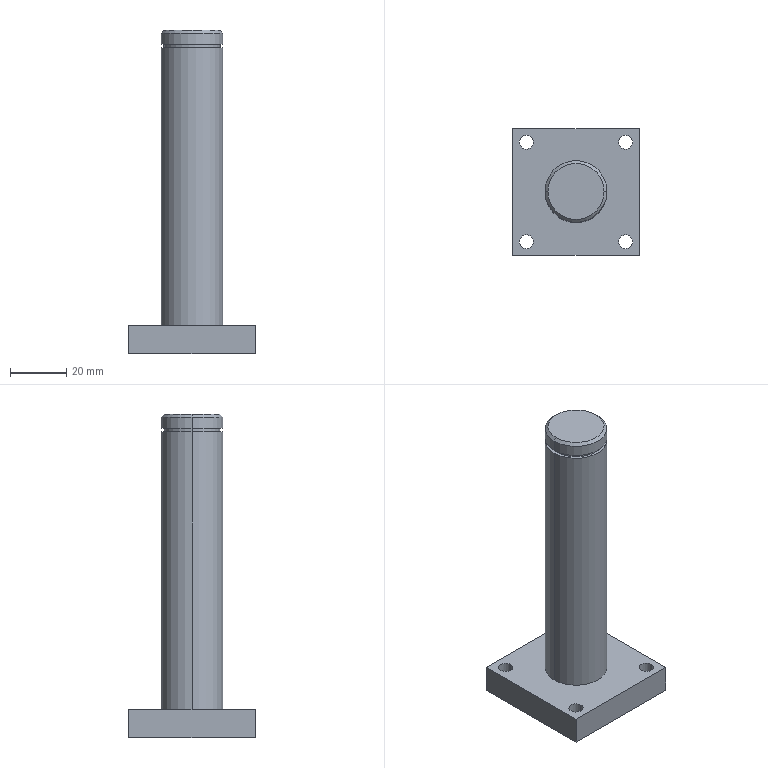Part | SolidWorks | features ICE 2, Chamfer 1, Extrusion 1 | 1 solid | 25 faces | box 45 x 45 x 115 mm | volume 59266 mm3 | cylinder 14 | plane 9 | cone 2 | commonest cylinder face diameters 5 x8 22 x4 20 x2
STEP:
#1=CARTESIAN_POINT('',(-11.,0.,114.));
#2=VERTEX_POINT('',#1);
#3=CARTESIAN_POINT('',(11.,0.,114.));
#4=VERTEX_POINT('',#3);
#5=CARTESIAN_POINT('',(0.,0.,114.));
#6=DIRECTION('',(0.,0.,-1.));
#7=DIRECTION('',(1.,0.,0.));
#8=AXIS2_PLACEMENT_3D('',#5,#6,#7);
#9=CIRCLE('',#8,11.);
#10=EDGE_CURVE('',#2,#4,#9,.T.);
#11=ORIENTED_EDGE('',*,*,#10,.T.);
#12=CARTESIAN_POINT('',(11.,0.,110.));
#13=VERTEX_POINT('',#12);
#14=CARTESIAN_POINT('',(11.,0.,115.));
#15=DIRECTION('',(0.,0.,-1.));
#16=VECTOR('',#15,1000.);
#17=LINE('',#14,#16);
#18=EDGE_CURVE('',#4,#13,#17,.T.);
#19=ORIENTED_EDGE('',*,*,#18,.T.);
#20=CARTESIAN_POINT('',(-11.,0.,110.));
#21=VERTEX_POINT('',#20);
#22=CARTESIAN_POINT('',(0.,0.,110.));
#23=DIRECTION('',(0.,0.,1.));
#24=DIRECTION('',(1.,0.,0.));
#25=AXIS2_PLACEMENT_3D('',#22,#23,#24);
#26=CIRCLE('',#25,11.);
#27=EDGE_CURVE('',#13,#21,#26,.T.);
#28=ORIENTED_EDGE('',*,*,#27,.T.);
#29=CARTESIAN_POINT('',(-11.,0.,115.));
#30=DIRECTION('',(0.,0.,-1.));
#31=VECTOR('',#30,1000.);
#32=LINE('',#29,#31);
#33=EDGE_CURVE('',#2,#21,#32,.T.);
#34=ORIENTED_EDGE('',*,*,#33,.F.);
#35=EDGE_LOOP('',(#11,#19,#28,#34));
#36=FACE_OUTER_BOUND('',#35,.T.);
#37=CARTESIAN_POINT('',(0.,0.,115.));
#38=DIRECTION('',(0.,0.,-1.));
#39=DIRECTION('',(-1.,0.,0.));
#40=AXIS2_PLACEMENT_3D('',#37,#38,#39);
#41=CYLINDRICAL_SURFACE('',#40,11.);
#42=ADVANCED_FACE('',(#36),#41,.T.);
#43=CARTESIAN_POINT('',(10.,0.,115.));
#44=VERTEX_POINT('',#43);
#45=CARTESIAN_POINT('',(-10.,0.,115.));
#46=VERTEX_POINT('',#45);
#47=CARTESIAN_POINT('',(0.,0.,115.));
#48=DIRECTION('',(0.,0.,1.));
#49=DIRECTION('',(1.,0.,0.));
#50=AXIS2_PLACEMENT_3D('',#47,#48,#49);
#51=CIRCLE('',#50,10.);
#52=EDGE_CURVE('',#44,#46,#51,.T.);
#53=ORIENTED_EDGE('',*,*,#52,.F.);
#54=CARTESIAN_POINT('',(10.,0.,115.));
#55=DIRECTION('',(0.7071,0.,-0.7071));
#56=VECTOR('',#55,1000.);
#57=LINE('',#54,#56);
#58=EDGE_CURVE('',#44,#4,#57,.T.);
#59=ORIENTED_EDGE('',*,*,#58,.T.);
#60=ORIENTED_EDGE('',*,*,#10,.F.);
#61=CARTESIAN_POINT('',(-10.,0.,115.));
#62=DIRECTION('',(-0.7071,0.,-0.7071));
#63=VECTOR('',#62,1000.);
#64=LINE('',#61,#63);
#65=EDGE_CURVE('',#46,#2,#64,.T.);
#66=ORIENTED_EDGE('',*,*,#65,.F.);
#67=EDGE_LOOP('',(#53,#59,#60,#66));
#68=FACE_OUTER_BOUND('',#67,.T.);
#69=CARTESIAN_POINT('',(0.,0.,115.));
#70=DIRECTION('',(0.,0.,-1.));
#71=DIRECTION('',(-1.,0.,0.));
#72=AXIS2_PLACEMENT_3D('',#69,#70,#71);
#73=CONICAL_SURFACE('',#72,10.,0.7854);
#74=ADVANCED_FACE('',(#68),#73,.T.);
#75=CARTESIAN_POINT('',(10.,0.,108.8));
#76=VERTEX_POINT('',#75);
#77=CARTESIAN_POINT('',(-10.,0.,108.8));
#78=VERTEX_POINT('',#77);
#79=CARTESIAN_POINT('',(0.,0.,108.8));
#80=DIRECTION('',(0.,0.,1.));
#81=DIRECTION('',(1.,0.,0.));
#82=AXIS2_PLACEMENT_3D('',#79,#80,#81);
#83=CIRCLE('',#82,10.);
#84=EDGE_CURVE('',#76,#78,#83,.T.);
#85=ORIENTED_EDGE('',*,*,#84,.T.);
#86=CARTESIAN_POINT('',(-10.,0.,110.));
#87=VERTEX_POINT('',#86);
#88=CARTESIAN_POINT('',(-10.,0.,108.8));
#89=DIRECTION('',(0.,0.,1.));
#90=VECTOR('',#89,1000.);
#91=LINE('',#88,#90);
#92=EDGE_CURVE('',#78,#87,#91,.T.);
#93=ORIENTED_EDGE('',*,*,#92,.T.);
#94=CARTESIAN_POINT('',(10.,0.,110.));
#95=VERTEX_POINT('',#94);
#96=CARTESIAN_POINT('',(0.,0.,110.));
#97=DIRECTION('',(0.,0.,1.));
#98=DIRECTION('',(1.,0.,0.));
#99=AXIS2_PLACEMENT_3D('',#96,#97,#98);
#100=CIRCLE('',#99,10.);
#101=EDGE_CURVE('',#95,#87,#100,.T.);
#102=ORIENTED_EDGE('',*,*,#101,.F.);
#103=CARTESIAN_POINT('',(10.,0.,108.8));
#104=DIRECTION('',(0.,0.,1.));
#105=VECTOR('',#104,1000.);
#106=LINE('',#103,#105);
#107=EDGE_CURVE('',#76,#95,#106,.T.);
#108=ORIENTED_EDGE('',*,*,#107,.F.);
#109=EDGE_LOOP('',(#85,#93,#102,#108));
#110=FACE_OUTER_BOUND('',#109,.T.);
#111=CARTESIAN_POINT('',(0.,0.,108.8));
#112=DIRECTION('',(0.,0.,1.));
#113=DIRECTION('',(1.,0.,0.));
#114=AXIS2_PLACEMENT_3D('',#111,#112,#113);
#115=CYLINDRICAL_SURFACE('',#114,10.);
#116=ADVANCED_FACE('',(#110),#115,.T.);
#117=CARTESIAN_POINT('',(-20.178,17.678,10.));
#118=VERTEX_POINT('',#117);
#119=CARTESIAN_POINT('',(-15.178,17.678,10.));
#120=VERTEX_POINT('',#119);
#121=CARTESIAN_POINT('',(-17.678,17.678,10.));
#122=DIRECTION('',(0.,0.,1.));
#123=DIRECTION('',(1.,0.,0.));
#124=AXIS2_PLACEMENT_3D('',#121,#122,#123);
#125=CIRCLE('',#124,2.5);
#126=EDGE_CURVE('',#118,#120,#125,.T.);
#127=ORIENTED_EDGE('',*,*,#126,.T.);
#128=CARTESIAN_POINT('',(-15.178,17.678,0.));
#129=VERTEX_POINT('',#128);
#130=CARTESIAN_POINT('',(-15.178,17.678,10.));
#131=DIRECTION('',(0.,0.,-1.));
#132=VECTOR('',#131,1000.);
#133=LINE('',#130,#132);
#134=EDGE_CURVE('',#120,#129,#133,.T.);
#135=ORIENTED_EDGE('',*,*,#134,.T.);
#136=CARTESIAN_POINT('',(-20.178,17.678,0.));
#137=VERTEX_POINT('',#136);
#138=CARTESIAN_POINT('',(-17.678,17.678,0.));
#139=DIRECTION('',(0.,0.,1.));
#140=DIRECTION('',(1.,0.,0.));
#141=AXIS2_PLACEMENT_3D('',#138,#139,#140);
#142=CIRCLE('',#141,2.5);
#143=EDGE_CURVE('',#137,#129,#142,.T.);
#144=ORIENTED_EDGE('',*,*,#143,.F.);
#145=CARTESIAN_POINT('',(-20.178,17.678,10.));
#146=DIRECTION('',(0.,0.,-1.));
#147=VECTOR('',#146,1000.);
#148=LINE('',#145,#147);
#149=EDGE_CURVE('',#118,#137,#148,.T.);
#150=ORIENTED_EDGE('',*,*,#149,.F.);
#151=EDGE_LOOP('',(#127,#135,#144,#150));
#152=FACE_OUTER_BOUND('',#151,.T.);
#153=CARTESIAN_POINT('',(-17.678,17.678,10.));
#154=DIRECTION('',(0.,0.,-1.));
#155=DIRECTION('',(-1.,0.,0.));
#156=AXIS2_PLACEMENT_3D('',#153,#154,#155);
#157=CYLINDRICAL_SURFACE('',#156,2.5);
#158=ADVANCED_FACE('',(#152),#157,.F.);
#159=CARTESIAN_POINT('',(-20.178,-17.678,10.));
#160=VERTEX_POINT('',#159);
#161=CARTESIAN_POINT('',(-15.178,-17.678,10.));
#162=VERTEX_POINT('',#161);
#163=CARTESIAN_POINT('',(-17.678,-17.678,10.));
#164=DIRECTION('',(0.,0.,1.));
#165=DIRECTION('',(1.,0.,0.));
#166=AXIS2_PLACEMENT_3D('',#163,#164,#165);
#167=CIRCLE('',#166,2.5);
#168=EDGE_CURVE('',#160,#162,#167,.T.);
#169=ORIENTED_EDGE('',*,*,#168,.T.);
#170=CARTESIAN_POINT('',(-15.178,-17.678,0.));
#171=VERTEX_POINT('',#170);
#172=CARTESIAN_POINT('',(-15.178,-17.678,10.));
#173=DIRECTION('',(0.,0.,-1.));
#174=VECTOR('',#173,1000.);
#175=LINE('',#172,#174);
#176=EDGE_CURVE('',#162,#171,#175,.T.);
#177=ORIENTED_EDGE('',*,*,#176,.T.);
#178=CARTESIAN_POINT('',(-20.178,-17.678,0.));
#179=VERTEX_POINT('',#178);
#180=CARTESIAN_POINT('',(-17.678,-17.678,0.));
#181=DIRECTION('',(0.,0.,1.));
#182=DIRECTION('',(1.,0.,0.));
#183=AXIS2_PLACEMENT_3D('',#180,#181,#182);
#184=CIRCLE('',#183,2.5);
#185=EDGE_CURVE('',#179,#171,#184,.T.);
#186=ORIENTED_EDGE('',*,*,#185,.F.);
#187=CARTESIAN_POINT('',(-20.178,-17.678,10.));
#188=DIRECTION('',(0.,0.,-1.));
#189=VECTOR('',#188,1000.);
#190=LINE('',#187,#189);
#191=EDGE_CURVE('',#160,#179,#190,.T.);
#192=ORIENTED_EDGE('',*,*,#191,.F.);
#193=EDGE_LOOP('',(#169,#177,#186,#192));
#194=FACE_OUTER_BOUND('',#193,.T.);
#195=CARTESIAN_POINT('',(-17.678,-17.678,10.));
#196=DIRECTION('',(0.,0.,-1.));
#197=DIRECTION('',(-1.,0.,0.));
#198=AXIS2_PLACEMENT_3D('',#195,#196,#197);
#199=CYLINDRICAL_SURFACE('',#198,2.5);
#200=ADVANCED_FACE('',(#194),#199,.F.);
#201=CARTESIAN_POINT('',(15.178,-17.678,10.));
#202=VERTEX_POINT('',#201);
#203=CARTESIAN_POINT('',(20.178,-17.678,10.));
#204=VERTEX_POINT('',#203);
#205=CARTESIAN_POINT('',(17.678,-17.678,10.));
#206=DIRECTION('',(0.,0.,1.));
#207=DIRECTION('',(1.,0.,0.));
#208=AXIS2_PLACEMENT_3D('',#205,#206,#207);
#209=CIRCLE('',#208,2.5);
#210=EDGE_CURVE('',#202,#204,#209,.T.);
#211=ORIENTED_EDGE('',*,*,#210,.T.);
#212=CARTESIAN_POINT('',(20.178,-17.678,0.));
#213=VERTEX_POINT('',#212);
#214=CARTESIAN_POINT('',(20.178,-17.678,10.));
#215=DIRECTION('',(0.,0.,-1.));
#216=VECTOR('',#215,1000.);
#217=LINE('',#214,#216);
#218=EDGE_CURVE('',#204,#213,#217,.T.);
#219=ORIENTED_EDGE('',*,*,#218,.T.);
#220=CARTESIAN_POINT('',(15.178,-17.678,0.));
#221=VERTEX_POINT('',#220);
#222=CARTESIAN_POINT('',(17.678,-17.678,0.));
#223=DIRECTION('',(0.,0.,1.));
#224=DIRECTION('',(1.,0.,0.));
#225=AXIS2_PLACEMENT_3D('',#222,#223,#224);
#226=CIRCLE('',#225,2.5);
#227=EDGE_CURVE('',#221,#213,#226,.T.);
#228=ORIENTED_EDGE('',*,*,#227,.F.);
#229=CARTESIAN_POINT('',(15.178,-17.678,10.));
#230=DIRECTION('',(0.,0.,-1.));
#231=VECTOR('',#230,1000.);
#232=LINE('',#229,#231);
#233=EDGE_CURVE('',#202,#221,#232,.T.);
#234=ORIENTED_EDGE('',*,*,#233,.F.);
#235=EDGE_LOOP('',(#211,#219,#228,#234));
#236=FACE_OUTER_BOUND('',#235,.T.);
#237=CARTESIAN_POINT('',(17.678,-17.678,10.));
#238=DIRECTION('',(0.,0.,-1.));
#239=DIRECTION('',(-1.,0.,0.));
#240=AXIS2_PLACEMENT_3D('',#237,#238,#239);
#241=CYLINDRICAL_SURFACE('',#240,2.5);
#242=ADVANCED_FACE('',(#236),#241,.F.);
#243=CARTESIAN_POINT('',(15.178,17.678,10.));
#244=VERTEX_POINT('',#243);
#245=CARTESIAN_POINT('',(20.178,17.678,10.));
#246=VERTEX_POINT('',#245);
#247=CARTESIAN_POINT('',(17.678,17.678,10.));
#248=DIRECTION('',(0.,0.,1.));
#249=DIRECTION('',(1.,0.,0.));
#250=AXIS2_PLACEMENT_3D('',#247,#248,#249);
#251=CIRCLE('',#250,2.5);
#252=EDGE_CURVE('',#244,#246,#251,.T.);
#253=ORIENTED_EDGE('',*,*,#252,.T.);
#254=CARTESIAN_POINT('',(20.178,17.678,0.));
#255=VERTEX_POINT('',#254);
#256=CARTESIAN_POINT('',(20.178,17.678,10.));
#257=DIRECTION('',(0.,0.,-1.));
#258=VECTOR('',#257,1000.);
#259=LINE('',#256,#258);
#260=EDGE_CURVE('',#246,#255,#259,.T.);
#261=ORIENTED_EDGE('',*,*,#260,.T.);
#262=CARTESIAN_POINT('',(15.178,17.678,0.));
#263=VERTEX_POINT('',#262);
#264=CARTESIAN_POINT('',(17.678,17.678,0.));
#265=DIRECTION('',(0.,0.,1.));
#266=DIRECTION('',(1.,0.,0.));
#267=AXIS2_PLACEMENT_3D('',#264,#265,#266);
#268=CIRCLE('',#267,2.5);
#269=EDGE_CURVE('',#263,#255,#268,.T.);
#270=ORIENTED_EDGE('',*,*,#269,.F.);
#271=CARTESIAN_POINT('',(15.178,17.678,10.));
#272=DIRECTION('',(0.,0.,-1.));
#273=VECTOR('',#272,1000.);
#274=LINE('',#271,#273);
#275=EDGE_CURVE('',#244,#263,#274,.T.);
#276=ORIENTED_EDGE('',*,*,#275,.F.);
#277=EDGE_LOOP('',(#253,#261,#270,#276));
#278=FACE_OUTER_BOUND('',#277,.T.);
#279=CARTESIAN_POINT('',(17.678,17.678,10.));
#280=DIRECTION('',(0.,0.,-1.));
#281=DIRECTION('',(-1.,0.,0.));
#282=AXIS2_PLACEMENT_3D('',#279,#280,#281);
#283=CYLINDRICAL_SURFACE('',#282,2.5);
#284=ADVANCED_FACE('',(#278),#283,.F.);
#285=CARTESIAN_POINT('',(11.,0.,108.8));
#286=VERTEX_POINT('',#285);
#287=CARTESIAN_POINT('',(-11.,0.,108.8));
#288=VERTEX_POINT('',#287);
#289=CARTESIAN_POINT('',(0.,0.,108.8));
#290=DIRECTION('',(0.,0.,1.));
#291=DIRECTION('',(1.,0.,0.));
#292=AXIS2_PLACEMENT_3D('',#289,#290,#291);
#293=CIRCLE('',#292,11.);
#294=EDGE_CURVE('',#286,#288,#293,.T.);
#295=ORIENTED_EDGE('',*,*,#294,.F.);
#296=CARTESIAN_POINT('',(11.,0.,10.));
#297=VERTEX_POINT('',#296);
#298=CARTESIAN_POINT('',(11.,0.,115.));
#299=DIRECTION('',(0.,0.,-1.));
#300=VECTOR('',#299,1000.);
#301=LINE('',#298,#300);
#302=EDGE_CURVE('',#286,#297,#301,.T.);
#303=ORIENTED_EDGE('',*,*,#302,.T.);
#304=CARTESIAN_POINT('',(-11.,0.,10.));
#305=VERTEX_POINT('',#304);
#306=CARTESIAN_POINT('',(0.,0.,10.));
#307=DIRECTION('',(0.,0.,1.));
#308=DIRECTION('',(1.,0.,0.));
#309=AXIS2_PLACEMENT_3D('',#306,#307,#308);
#310=CIRCLE('',#309,11.);
#311=EDGE_CURVE('',#297,#305,#310,.T.);
#312=ORIENTED_EDGE('',*,*,#311,.T.);
#313=CARTESIAN_POINT('',(-11.,0.,115.));
#314=DIRECTION('',(0.,0.,-1.));
#315=VECTOR('',#314,1000.);
#316=LINE('',#313,#315);
#317=EDGE_CURVE('',#288,#305,#316,.T.);
#318=ORIENTED_EDGE('',*,*,#317,.F.);
#319=EDGE_LOOP('',(#295,#303,#312,#318));
#320=FACE_OUTER_BOUND('',#319,.T.);
#321=CARTESIAN_POINT('',(0.,0.,115.));
#322=DIRECTION('',(0.,0.,-1.));
#323=DIRECTION('',(-1.,0.,0.));
#324=AXIS2_PLACEMENT_3D('',#321,#322,#323);
#325=CYLINDRICAL_SURFACE('',#324,11.);
#326=ADVANCED_FACE('',(#320),#325,.T.);
#327=ORIENTED_EDGE('',*,*,#302,.F.);
#328=CARTESIAN_POINT('',(0.,0.,108.8));
#329=DIRECTION('',(0.,0.,1.));
#330=DIRECTION('',(1.,0.,0.));
#331=AXIS2_PLACEMENT_3D('',#328,#329,#330);
#332=CIRCLE('',#331,11.);
#333=EDGE_CURVE('',#288,#286,#332,.T.);
#334=ORIENTED_EDGE('',*,*,#333,.F.);
#335=ORIENTED_EDGE('',*,*,#317,.T.);
#336=CARTESIAN_POINT('',(0.,0.,10.));
#337=DIRECTION('',(0.,0.,1.));
#338=DIRECTION('',(1.,0.,0.));
#339=AXIS2_PLACEMENT_3D('',#336,#337,#338);
#340=CIRCLE('',#339,11.);
#341=EDGE_CURVE('',#305,#297,#340,.T.);
#342=ORIENTED_EDGE('',*,*,#341,.T.);
#343=EDGE_LOOP('',(#327,#334,#335,#342));
#344=FACE_OUTER_BOUND('',#343,.T.);
#345=CARTESIAN_POINT('',(0.,0.,115.));
#346=DIRECTION('',(0.,0.,-1.));
#347=DIRECTION('',(-1.,0.,0.));
#348=AXIS2_PLACEMENT_3D('',#345,#346,#347);
#349=CYLINDRICAL_SURFACE('',#348,11.);
#350=ADVANCED_FACE('',(#344),#349,.T.);
#351=ORIENTED_EDGE('',*,*,#341,.F.);
#352=ORIENTED_EDGE('',*,*,#311,.F.);
#353=EDGE_LOOP('',(#351,#352));
#354=FACE_BOUND('',#353,.T.);
#355=ORIENTED_EDGE('',*,*,#168,.F.);
#356=CARTESIAN_POINT('',(-17.678,-17.678,10.));
#357=DIRECTION('',(0.,0.,1.));
#358=DIRECTION('',(1.,0.,0.));
#359=AXIS2_PLACEMENT_3D('',#356,#357,#358);
#360=CIRCLE('',#359,2.5);
#361=EDGE_CURVE('',#162,#160,#360,.T.);
#362=ORIENTED_EDGE('',*,*,#361,.F.);
#363=EDGE_LOOP('',(#355,#362));
#364=FACE_BOUND('',#363,.T.);
#365=ORIENTED_EDGE('',*,*,#252,.F.);
#366=CARTESIAN_POINT('',(17.678,17.678,10.));
#367=DIRECTION('',(0.,0.,1.));
#368=DIRECTION('',(1.,0.,0.));
#369=AXIS2_PLACEMENT_3D('',#366,#367,#368);
#370=CIRCLE('',#369,2.5);
#371=EDGE_CURVE('',#246,#244,#370,.T.);
#372=ORIENTED_EDGE('',*,*,#371,.F.);
#373=EDGE_LOOP('',(#365,#372));
#374=FACE_BOUND('',#373,.T.);
#375=CARTESIAN_POINT('',(22.5,-22.5,10.));
#376=VERTEX_POINT('',#375);
#377=CARTESIAN_POINT('',(22.5,22.5,10.));
#378=VERTEX_POINT('',#377);
#379=CARTESIAN_POINT('',(22.5,22.5,10.));
#380=DIRECTION('',(0.,1.,0.));
#381=VECTOR('',#380,1000.);
#382=LINE('',#379,#381);
#383=EDGE_CURVE('',#376,#378,#382,.T.);
#384=ORIENTED_EDGE('',*,*,#383,.T.);
#385=CARTESIAN_POINT('',(-22.5,22.5,10.));
#386=VERTEX_POINT('',#385);
#387=CARTESIAN_POINT('',(-22.5,22.5,10.));
#388=DIRECTION('',(-1.,0.,0.));
#389=VECTOR('',#388,1000.);
#390=LINE('',#387,#389);
#391=EDGE_CURVE('',#378,#386,#390,.T.);
#392=ORIENTED_EDGE('',*,*,#391,.T.);
#393=CARTESIAN_POINT('',(-22.5,-22.5,10.));
#394=VERTEX_POINT('',#393);
#395=CARTESIAN_POINT('',(-22.5,22.5,10.));
#396=DIRECTION('',(0.,-1.,0.));
#397=VECTOR('',#396,1000.);
#398=LINE('',#395,#397);
#399=EDGE_CURVE('',#386,#394,#398,.T.);
#400=ORIENTED_EDGE('',*,*,#399,.T.);
#401=CARTESIAN_POINT('',(-22.5,-22.5,10.));
#402=DIRECTION('',(1.,0.,0.));
#403=VECTOR('',#402,1000.);
#404=LINE('',#401,#403);
#405=EDGE_CURVE('',#394,#376,#404,.T.);
#406=ORIENTED_EDGE('',*,*,#405,.T.);
#407=EDGE_LOOP('',(#384,#392,#400,#406));
#408=FACE_OUTER_BOUND('',#407,.T.);
#409=ORIENTED_EDGE('',*,*,#210,.F.);
#410=CARTESIAN_POINT('',(17.678,-17.678,10.));
#411=DIRECTION('',(0.,0.,1.));
#412=DIRECTION('',(1.,0.,0.));
#413=AXIS2_PLACEMENT_3D('',#410,#411,#412);
#414=CIRCLE('',#413,2.5);
#415=EDGE_CURVE('',#204,#202,#414,.T.);
#416=ORIENTED_EDGE('',*,*,#415,.F.);
#417=EDGE_LOOP('',(#409,#416));
#418=FACE_BOUND('',#417,.T.);
#419=ORIENTED_EDGE('',*,*,#126,.F.);
#420=CARTESIAN_POINT('',(-17.678,17.678,10.));
#421=DIRECTION('',(0.,0.,1.));
#422=DIRECTION('',(1.,0.,0.));
#423=AXIS2_PLACEMENT_3D('',#420,#421,#422);
#424=CIRCLE('',#423,2.5);
#425=EDGE_CURVE('',#120,#118,#424,.T.);
#426=ORIENTED_EDGE('',*,*,#425,.F.);
#427=EDGE_LOOP('',(#419,#426));
#428=FACE_BOUND('',#427,.T.);
#429=CARTESIAN_POINT('',(0.,0.,10.));
#430=DIRECTION('',(0.,0.,1.));
#431=DIRECTION('',(1.,0.,0.));
#432=AXIS2_PLACEMENT_3D('',#429,#430,#431);
#433=PLANE('',#432);
#434=ADVANCED_FACE('',(#354,#364,#374,#408,#418,#428),#433,.T.);
#435=CARTESIAN_POINT('',(22.5,-22.5,0.));
#436=VERTEX_POINT('',#435);
#437=CARTESIAN_POINT('',(22.5,22.5,0.));
#438=VERTEX_POINT('',#437);
#439=CARTESIAN_POINT('',(22.5,22.5,0.));
#440=DIRECTION('',(0.,1.,0.));
#441=VECTOR('',#440,1000.);
#442=LINE('',#439,#441);
#443=EDGE_CURVE('',#436,#438,#442,.T.);
#444=ORIENTED_EDGE('',*,*,#443,.F.);
#445=CARTESIAN_POINT('',(-22.5,-22.5,0.));
#446=VERTEX_POINT('',#445);
#447=CARTESIAN_POINT('',(-22.5,-22.5,0.));
#448=DIRECTION('',(1.,0.,0.));
#449=VECTOR('',#448,1000.);
#450=LINE('',#447,#449);
#451=EDGE_CURVE('',#446,#436,#450,.T.);
#452=ORIENTED_EDGE('',*,*,#451,.F.);
#453=CARTESIAN_POINT('',(-22.5,22.5,0.));
#454=VERTEX_POINT('',#453);
#455=CARTESIAN_POINT('',(-22.5,22.5,0.));
#456=DIRECTION('',(0.,-1.,0.));
#457=VECTOR('',#456,1000.);
#458=LINE('',#455,#457);
#459=EDGE_CURVE('',#454,#446,#458,.T.);
#460=ORIENTED_EDGE('',*,*,#459,.F.);
#461=CARTESIAN_POINT('',(-22.5,22.5,0.));
#462=DIRECTION('',(-1.,0.,0.));
#463=VECTOR('',#462,1000.);
#464=LINE('',#461,#463);
#465=EDGE_CURVE('',#438,#454,#464,.T.);
#466=ORIENTED_EDGE('',*,*,#465,.F.);
#467=EDGE_LOOP('',(#444,#452,#460,#466));
#468=FACE_OUTER_BOUND('',#467,.T.);
#469=ORIENTED_EDGE('',*,*,#269,.T.);
#470=CARTESIAN_POINT('',(17.678,17.678,0.));
#471=DIRECTION('',(0.,0.,1.));
#472=DIRECTION('',(1.,0.,0.));
#473=AXIS2_PLACEMENT_3D('',#470,#471,#472);
#474=CIRCLE('',#473,2.5);
#475=EDGE_CURVE('',#255,#263,#474,.T.);
#476=ORIENTED_EDGE('',*,*,#475,.T.);
#477=EDGE_LOOP('',(#469,#476));
#478=FACE_BOUND('',#477,.T.);
#479=ORIENTED_EDGE('',*,*,#227,.T.);
#480=CARTESIAN_POINT('',(17.678,-17.678,0.));
#481=DIRECTION('',(0.,0.,1.));
#482=DIRECTION('',(1.,0.,0.));
#483=AXIS2_PLACEMENT_3D('',#480,#481,#482);
#484=CIRCLE('',#483,2.5);
#485=EDGE_CURVE('',#213,#221,#484,.T.);
#486=ORIENTED_EDGE('',*,*,#485,.T.);
#487=EDGE_LOOP('',(#479,#486));
#488=FACE_BOUND('',#487,.T.);
#489=ORIENTED_EDGE('',*,*,#185,.T.);
#490=CARTESIAN_POINT('',(-17.678,-17.678,0.));
#491=DIRECTION('',(0.,0.,1.));
#492=DIRECTION('',(1.,0.,0.));
#493=AXIS2_PLACEMENT_3D('',#490,#491,#492);
#494=CIRCLE('',#493,2.5);
#495=EDGE_CURVE('',#171,#179,#494,.T.);
#496=ORIENTED_EDGE('',*,*,#495,.T.);
#497=EDGE_LOOP('',(#489,#496));
#498=FACE_BOUND('',#497,.T.);
#499=ORIENTED_EDGE('',*,*,#143,.T.);
#500=CARTESIAN_POINT('',(-17.678,17.678,0.));
#501=DIRECTION('',(0.,0.,1.));
#502=DIRECTION('',(1.,0.,0.));
#503=AXIS2_PLACEMENT_3D('',#500,#501,#502);
#504=CIRCLE('',#503,2.5);
#505=EDGE_CURVE('',#129,#137,#504,.T.);
#506=ORIENTED_EDGE('',*,*,#505,.T.);
#507=EDGE_LOOP('',(#499,#506));
#508=FACE_BOUND('',#507,.T.);
#509=CARTESIAN_POINT('',(0.,0.,0.));
#510=DIRECTION('',(0.,0.,1.));
#511=DIRECTION('',(1.,0.,0.));
#512=AXIS2_PLACEMENT_3D('',#509,#510,#511);
#513=PLANE('',#512);
#514=ADVANCED_FACE('',(#468,#478,#488,#498,#508),#513,.F.);
#515=ORIENTED_EDGE('',*,*,#443,.T.);
#516=CARTESIAN_POINT('',(22.5,22.5,10.));
#517=DIRECTION('',(0.,0.,-1.));
#518=VECTOR('',#517,1000.);
#519=LINE('',#516,#518);
#520=EDGE_CURVE('',#378,#438,#519,.T.);
#521=ORIENTED_EDGE('',*,*,#520,.F.);
#522=ORIENTED_EDGE('',*,*,#383,.F.);
#523=CARTESIAN_POINT('',(22.5,-22.5,10.));
#524=DIRECTION('',(0.,0.,-1.));
#525=VECTOR('',#524,1000.);
#526=LINE('',#523,#525);
#527=EDGE_CURVE('',#376,#436,#526,.T.);
#528=ORIENTED_EDGE('',*,*,#527,.T.);
#529=EDGE_LOOP('',(#515,#521,#522,#528));
#530=FACE_OUTER_BOUND('',#529,.T.);
#531=CARTESIAN_POINT('',(22.5,22.5,10.));
#532=DIRECTION('',(-1.,0.,0.));
#533=DIRECTION('',(0.,-1.,0.));
#534=AXIS2_PLACEMENT_3D('',#531,#532,#533);
#535=PLANE('',#534);
#536=ADVANCED_FACE('',(#530),#535,.F.);
#537=ORIENTED_EDGE('',*,*,#465,.T.);
#538=CARTESIAN_POINT('',(-22.5,22.5,10.));
#539=DIRECTION('',(0.,0.,-1.));
#540=VECTOR('',#539,1000.);
#541=LINE('',#538,#540);
#542=EDGE_CURVE('',#386,#454,#541,.T.);
#543=ORIENTED_EDGE('',*,*,#542,.F.);
#544=ORIENTED_EDGE('',*,*,#391,.F.);
#545=ORIENTED_EDGE('',*,*,#520,.T.);
#546=EDGE_LOOP('',(#537,#543,#544,#545));
#547=FACE_OUTER_BOUND('',#546,.T.);
#548=CARTESIAN_POINT('',(-22.5,22.5,10.));
#549=DIRECTION('',(0.,-1.,0.));
#550=DIRECTION('',(0.,0.,-1.));
#551=AXIS2_PLACEMENT_3D('',#548,#549,#550);
#552=PLANE('',#551);
#553=ADVANCED_FACE('',(#547),#552,.F.);
#554=ORIENTED_EDGE('',*,*,#459,.T.);
#555=CARTESIAN_POINT('',(-22.5,-22.5,10.));
#556=DIRECTION('',(0.,0.,-1.));
#557=VECTOR('',#556,1000.);
#558=LINE('',#555,#557);
#559=EDGE_CURVE('',#394,#446,#558,.T.);
#560=ORIENTED_EDGE('',*,*,#559,.F.);
#561=ORIENTED_EDGE('',*,*,#399,.F.);
#562=ORIENTED_EDGE('',*,*,#542,.T.);
#563=EDGE_LOOP('',(#554,#560,#561,#562));
#564=FACE_OUTER_BOUND('',#563,.T.);
#565=CARTESIAN_POINT('',(-22.5,22.5,10.));
#566=DIRECTION('',(1.,0.,0.));
#567=DIRECTION('',(0.,1.,0.));
#568=AXIS2_PLACEMENT_3D('',#565,#566,#567);
#569=PLANE('',#568);
#570=ADVANCED_FACE('',(#564),#569,.F.);
#571=ORIENTED_EDGE('',*,*,#451,.T.);
#572=ORIENTED_EDGE('',*,*,#527,.F.);
#573=ORIENTED_EDGE('',*,*,#405,.F.);
#574=ORIENTED_EDGE('',*,*,#559,.T.);
#575=EDGE_LOOP('',(#571,#572,#573,#574));
#576=FACE_OUTER_BOUND('',#575,.T.);
#577=CARTESIAN_POINT('',(-22.5,-22.5,10.));
#578=DIRECTION('',(0.,1.,0.));
#579=DIRECTION('',(0.,0.,1.));
#580=AXIS2_PLACEMENT_3D('',#577,#578,#579);
#581=PLANE('',#580);
#582=ADVANCED_FACE('',(#576),#581,.F.);
#583=ORIENTED_EDGE('',*,*,#260,.F.);
#584=ORIENTED_EDGE('',*,*,#371,.T.);
#585=ORIENTED_EDGE('',*,*,#275,.T.);
#586=ORIENTED_EDGE('',*,*,#475,.F.);
#587=EDGE_LOOP('',(#583,#584,#585,#586));
#588=FACE_OUTER_BOUND('',#587,.T.);
#589=CARTESIAN_POINT('',(17.678,17.678,10.));
#590=DIRECTION('',(0.,0.,-1.));
#591=DIRECTION('',(-1.,0.,0.));
#592=AXIS2_PLACEMENT_3D('',#589,#590,#591);
#593=CYLINDRICAL_SURFACE('',#592,2.5);
#594=ADVANCED_FACE('',(#588),#593,.F.);
#595=ORIENTED_EDGE('',*,*,#218,.F.);
#596=ORIENTED_EDGE('',*,*,#415,.T.);
#597=ORIENTED_EDGE('',*,*,#233,.T.);
#598=ORIENTED_EDGE('',*,*,#485,.F.);
#599=EDGE_LOOP('',(#595,#596,#597,#598));
#600=FACE_OUTER_BOUND('',#599,.T.);
#601=CARTESIAN_POINT('',(17.678,-17.678,10.));
#602=DIRECTION('',(0.,0.,-1.));
#603=DIRECTION('',(-1.,0.,0.));
#604=AXIS2_PLACEMENT_3D('',#601,#602,#603);
#605=CYLINDRICAL_SURFACE('',#604,2.5);
#606=ADVANCED_FACE('',(#600),#605,.F.);
#607=ORIENTED_EDGE('',*,*,#176,.F.);
#608=ORIENTED_EDGE('',*,*,#361,.T.);
#609=ORIENTED_EDGE('',*,*,#191,.T.);
#610=ORIENTED_EDGE('',*,*,#495,.F.);
#611=EDGE_LOOP('',(#607,#608,#609,#610));
#612=FACE_OUTER_BOUND('',#611,.T.);
#613=CARTESIAN_POINT('',(-17.678,-17.678,10.));
#614=DIRECTION('',(0.,0.,-1.));
#615=DIRECTION('',(-1.,0.,0.));
#616=AXIS2_PLACEMENT_3D('',#613,#614,#615);
#617=CYLINDRICAL_SURFACE('',#616,2.5);
#618=ADVANCED_FACE('',(#612),#617,.F.);
#619=ORIENTED_EDGE('',*,*,#134,.F.);
#620=ORIENTED_EDGE('',*,*,#425,.T.);
#621=ORIENTED_EDGE('',*,*,#149,.T.);
#622=ORIENTED_EDGE('',*,*,#505,.F.);
#623=EDGE_LOOP('',(#619,#620,#621,#622));
#624=FACE_OUTER_BOUND('',#623,.T.);
#625=CARTESIAN_POINT('',(-17.678,17.678,10.));
#626=DIRECTION('',(0.,0.,-1.));
#627=DIRECTION('',(-1.,0.,0.));
#628=AXIS2_PLACEMENT_3D('',#625,#626,#627);
#629=CYLINDRICAL_SURFACE('',#628,2.5);
#630=ADVANCED_FACE('',(#624),#629,.F.);
#631=ORIENTED_EDGE('',*,*,#84,.F.);
#632=CARTESIAN_POINT('',(0.,0.,108.8));
#633=DIRECTION('',(0.,0.,1.));
#634=DIRECTION('',(1.,0.,0.));
#635=AXIS2_PLACEMENT_3D('',#632,#633,#634);
#636=CIRCLE('',#635,10.);
#637=EDGE_CURVE('',#78,#76,#636,.T.);
#638=ORIENTED_EDGE('',*,*,#637,.F.);
#639=EDGE_LOOP('',(#631,#638));
#640=FACE_BOUND('',#639,.T.);
#641=ORIENTED_EDGE('',*,*,#333,.T.);
#642=ORIENTED_EDGE('',*,*,#294,.T.);
#643=EDGE_LOOP('',(#641,#642));
#644=FACE_OUTER_BOUND('',#643,.T.);
#645=CARTESIAN_POINT('',(0.,0.,108.8));
#646=DIRECTION('',(0.,0.,1.));
#647=DIRECTION('',(1.,0.,0.));
#648=AXIS2_PLACEMENT_3D('',#645,#646,#647);
#649=PLANE('',#648);
#650=ADVANCED_FACE('',(#640,#644),#649,.T.);
#651=ORIENTED_EDGE('',*,*,#101,.T.);
#652=CARTESIAN_POINT('',(0.,0.,110.));
#653=DIRECTION('',(0.,0.,1.));
#654=DIRECTION('',(1.,0.,0.));
#655=AXIS2_PLACEMENT_3D('',#652,#653,#654);
#656=CIRCLE('',#655,10.);
#657=EDGE_CURVE('',#87,#95,#656,.T.);
#658=ORIENTED_EDGE('',*,*,#657,.T.);
#659=EDGE_LOOP('',(#651,#658));
#660=FACE_BOUND('',#659,.T.);
#661=CARTESIAN_POINT('',(0.,0.,110.));
#662=DIRECTION('',(0.,0.,1.));
#663=DIRECTION('',(1.,0.,0.));
#664=AXIS2_PLACEMENT_3D('',#661,#662,#663);
#665=CIRCLE('',#664,11.);
#666=EDGE_CURVE('',#21,#13,#665,.T.);
#667=ORIENTED_EDGE('',*,*,#666,.F.);
#668=ORIENTED_EDGE('',*,*,#27,.F.);
#669=EDGE_LOOP('',(#667,#668));
#670=FACE_OUTER_BOUND('',#669,.T.);
#671=CARTESIAN_POINT('',(0.,0.,110.));
#672=DIRECTION('',(0.,0.,1.));
#673=DIRECTION('',(1.,0.,0.));
#674=AXIS2_PLACEMENT_3D('',#671,#672,#673);
#675=PLANE('',#674);
#676=ADVANCED_FACE('',(#660,#670),#675,.F.);
#677=ORIENTED_EDGE('',*,*,#92,.F.);
#678=ORIENTED_EDGE('',*,*,#637,.T.);
#679=ORIENTED_EDGE('',*,*,#107,.T.);
#680=ORIENTED_EDGE('',*,*,#657,.F.);
#681=EDGE_LOOP('',(#677,#678,#679,#680));
#682=FACE_OUTER_BOUND('',#681,.T.);
#683=CARTESIAN_POINT('',(0.,0.,108.8));
#684=DIRECTION('',(0.,0.,1.));
#685=DIRECTION('',(1.,0.,0.));
#686=AXIS2_PLACEMENT_3D('',#683,#684,#685);
#687=CYLINDRICAL_SURFACE('',#686,10.);
#688=ADVANCED_FACE('',(#682),#687,.T.);
#689=CARTESIAN_POINT('',(0.,0.,115.));
#690=DIRECTION('',(0.,0.,1.));
#691=DIRECTION('',(1.,0.,0.));
#692=AXIS2_PLACEMENT_3D('',#689,#690,#691);
#693=CIRCLE('',#692,10.);
#694=EDGE_CURVE('',#46,#44,#693,.T.);
#695=ORIENTED_EDGE('',*,*,#694,.T.);
#696=ORIENTED_EDGE('',*,*,#52,.T.);
#697=EDGE_LOOP('',(#695,#696));
#698=FACE_OUTER_BOUND('',#697,.T.);
#699=CARTESIAN_POINT('',(0.,0.,115.));
#700=DIRECTION('',(0.,0.,1.));
#701=DIRECTION('',(1.,0.,0.));
#702=AXIS2_PLACEMENT_3D('',#699,#700,#701);
#703=PLANE('',#702);
#704=ADVANCED_FACE('',(#698),#703,.T.);
#705=ORIENTED_EDGE('',*,*,#58,.F.);
#706=ORIENTED_EDGE('',*,*,#694,.F.);
#707=ORIENTED_EDGE('',*,*,#65,.T.);
#708=CARTESIAN_POINT('',(0.,0.,114.));
#709=DIRECTION('',(0.,0.,-1.));
#710=DIRECTION('',(1.,0.,0.));
#711=AXIS2_PLACEMENT_3D('',#708,#709,#710);
#712=CIRCLE('',#711,11.);
#713=EDGE_CURVE('',#4,#2,#712,.T.);
#714=ORIENTED_EDGE('',*,*,#713,.F.);
#715=EDGE_LOOP('',(#705,#706,#707,#714));
#716=FACE_OUTER_BOUND('',#715,.T.);
#717=CARTESIAN_POINT('',(0.,0.,115.));
#718=DIRECTION('',(0.,0.,-1.));
#719=DIRECTION('',(-1.,0.,0.));
#720=AXIS2_PLACEMENT_3D('',#717,#718,#719);
#721=CONICAL_SURFACE('',#720,10.,0.7854);
#722=ADVANCED_FACE('',(#716),#721,.T.);
#723=ORIENTED_EDGE('',*,*,#18,.F.);
#724=ORIENTED_EDGE('',*,*,#713,.T.);
#725=ORIENTED_EDGE('',*,*,#33,.T.);
#726=ORIENTED_EDGE('',*,*,#666,.T.);
#727=EDGE_LOOP('',(#723,#724,#725,#726));
#728=FACE_OUTER_BOUND('',#727,.T.);
#729=CARTESIAN_POINT('',(0.,0.,115.));
#730=DIRECTION('',(0.,0.,-1.));
#731=DIRECTION('',(-1.,0.,0.));
#732=AXIS2_PLACEMENT_3D('',#729,#730,#731);
#733=CYLINDRICAL_SURFACE('',#732,11.);
#734=ADVANCED_FACE('',(#728),#733,.T.);
#735=CLOSED_SHELL('',(#42,#74,#116,#158,#200,#242,#284,#326,#350,#434,#514,#536,#553,#570,#582,#594,#606,#618,#630,#650,#676,#688,#704,#722,#734));
#736=MANIFOLD_SOLID_BREP('',#735);
#737=CARTESIAN_POINT('',(0.,0.,0.));
#738=DIRECTION('',(0.,0.,1.));
#739=DIRECTION('',(1.,0.,0.));
#740=AXIS2_PLACEMENT_3D('',#737,#738,#739);
#741=(LENGTH_UNIT()NAMED_UNIT(*)SI_UNIT(.MILLI.,.METRE.));
#742=UNCERTAINTY_MEASURE_WITH_UNIT(LENGTH_MEASURE(0.00001),#741,'','');
#743=(NAMED_UNIT(*)PLANE_ANGLE_UNIT()SI_UNIT($,.RADIAN.));
#744=(NAMED_UNIT(*)SI_UNIT($,.STERADIAN.)SOLID_ANGLE_UNIT());
#745=(GEOMETRIC_REPRESENTATION_CONTEXT(3)GLOBAL_UNCERTAINTY_ASSIGNED_CONTEXT((#742))GLOBAL_UNIT_ASSIGNED_CONTEXT((#741,#743,#744))REPRESENTATION_CONTEXT('',''));
#746=ADVANCED_BREP_SHAPE_REPRESENTATION('',(#736,#740),#745);